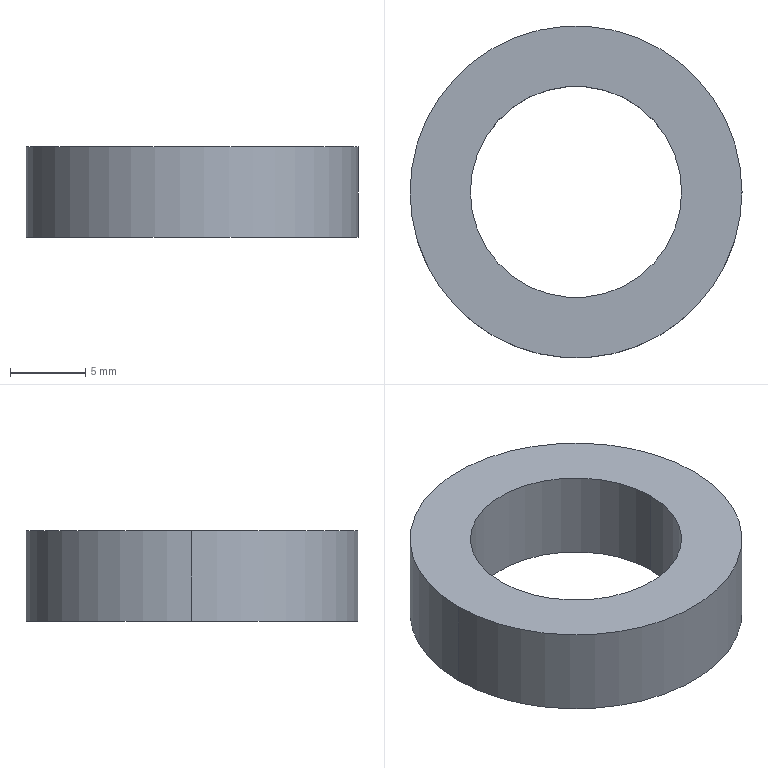Part | SolidWorks | features Revolution 1 | 1 solid | 6 faces | box 22 x 22 x 6 mm | volume 1357 mm3 | cylinder 4 | plane 2 | commonest cylinder face diameters 14 x2 22 x2
STEP:
#1=CARTESIAN_POINT('',(11.,0.,-6.));
#2=VERTEX_POINT('',#1);
#3=CARTESIAN_POINT('',(-11.,0.,-6.));
#4=VERTEX_POINT('',#3);
#5=CARTESIAN_POINT('',(0.,0.,-6.));
#6=DIRECTION('',(0.,0.,1.));
#7=DIRECTION('',(1.,0.,0.));
#8=AXIS2_PLACEMENT_3D('',#5,#6,#7);
#9=CIRCLE('',#8,11.);
#10=EDGE_CURVE('',#2,#4,#9,.T.);
#11=ORIENTED_EDGE('',*,*,#10,.T.);
#12=CARTESIAN_POINT('',(-11.,0.,0.));
#13=VERTEX_POINT('',#12);
#14=CARTESIAN_POINT('',(-11.,0.,4.548));
#15=DIRECTION('',(0.,0.,1.));
#16=VECTOR('',#15,1000.);
#17=LINE('',#14,#16);
#18=EDGE_CURVE('',#4,#13,#17,.T.);
#19=ORIENTED_EDGE('',*,*,#18,.T.);
#20=CARTESIAN_POINT('',(11.,0.,0.));
#21=VERTEX_POINT('',#20);
#22=CARTESIAN_POINT('',(0.,0.,0.));
#23=DIRECTION('',(0.,0.,1.));
#24=DIRECTION('',(1.,0.,0.));
#25=AXIS2_PLACEMENT_3D('',#22,#23,#24);
#26=CIRCLE('',#25,11.);
#27=EDGE_CURVE('',#21,#13,#26,.T.);
#28=ORIENTED_EDGE('',*,*,#27,.F.);
#29=CARTESIAN_POINT('',(11.,0.,4.548));
#30=DIRECTION('',(0.,0.,1.));
#31=VECTOR('',#30,1000.);
#32=LINE('',#29,#31);
#33=EDGE_CURVE('',#2,#21,#32,.T.);
#34=ORIENTED_EDGE('',*,*,#33,.F.);
#35=EDGE_LOOP('',(#11,#19,#28,#34));
#36=FACE_OUTER_BOUND('',#35,.T.);
#37=CARTESIAN_POINT('',(0.,0.,4.548));
#38=DIRECTION('',(0.,0.,1.));
#39=DIRECTION('',(1.,0.,0.));
#40=AXIS2_PLACEMENT_3D('',#37,#38,#39);
#41=CYLINDRICAL_SURFACE('',#40,11.);
#42=ADVANCED_FACE('',(#36),#41,.T.);
#43=CARTESIAN_POINT('',(-7.,0.,-6.));
#44=VERTEX_POINT('',#43);
#45=CARTESIAN_POINT('',(7.,0.,-6.));
#46=VERTEX_POINT('',#45);
#47=CARTESIAN_POINT('',(0.,0.,-6.));
#48=DIRECTION('',(0.,0.,1.));
#49=DIRECTION('',(1.,0.,0.));
#50=AXIS2_PLACEMENT_3D('',#47,#48,#49);
#51=CIRCLE('',#50,7.);
#52=EDGE_CURVE('',#44,#46,#51,.T.);
#53=ORIENTED_EDGE('',*,*,#52,.F.);
#54=CARTESIAN_POINT('',(-7.,0.,0.));
#55=VERTEX_POINT('',#54);
#56=CARTESIAN_POINT('',(-7.,0.,4.548));
#57=DIRECTION('',(0.,0.,1.));
#58=VECTOR('',#57,1000.);
#59=LINE('',#56,#58);
#60=EDGE_CURVE('',#44,#55,#59,.T.);
#61=ORIENTED_EDGE('',*,*,#60,.T.);
#62=CARTESIAN_POINT('',(7.,0.,0.));
#63=VERTEX_POINT('',#62);
#64=CARTESIAN_POINT('',(0.,0.,0.));
#65=DIRECTION('',(0.,0.,1.));
#66=DIRECTION('',(1.,0.,0.));
#67=AXIS2_PLACEMENT_3D('',#64,#65,#66);
#68=CIRCLE('',#67,7.);
#69=EDGE_CURVE('',#55,#63,#68,.T.);
#70=ORIENTED_EDGE('',*,*,#69,.T.);
#71=CARTESIAN_POINT('',(7.,0.,4.548));
#72=DIRECTION('',(0.,0.,1.));
#73=VECTOR('',#72,1000.);
#74=LINE('',#71,#73);
#75=EDGE_CURVE('',#46,#63,#74,.T.);
#76=ORIENTED_EDGE('',*,*,#75,.F.);
#77=EDGE_LOOP('',(#53,#61,#70,#76));
#78=FACE_OUTER_BOUND('',#77,.T.);
#79=CARTESIAN_POINT('',(0.,0.,4.548));
#80=DIRECTION('',(0.,0.,1.));
#81=DIRECTION('',(1.,0.,0.));
#82=AXIS2_PLACEMENT_3D('',#79,#80,#81);
#83=CYLINDRICAL_SURFACE('',#82,7.);
#84=ADVANCED_FACE('',(#78),#83,.F.);
#85=ORIENTED_EDGE('',*,*,#60,.F.);
#86=CARTESIAN_POINT('',(0.,0.,-6.));
#87=DIRECTION('',(0.,0.,1.));
#88=DIRECTION('',(1.,0.,0.));
#89=AXIS2_PLACEMENT_3D('',#86,#87,#88);
#90=CIRCLE('',#89,7.);
#91=EDGE_CURVE('',#46,#44,#90,.T.);
#92=ORIENTED_EDGE('',*,*,#91,.F.);
#93=ORIENTED_EDGE('',*,*,#75,.T.);
#94=CARTESIAN_POINT('',(0.,0.,0.));
#95=DIRECTION('',(0.,0.,1.));
#96=DIRECTION('',(1.,0.,0.));
#97=AXIS2_PLACEMENT_3D('',#94,#95,#96);
#98=CIRCLE('',#97,7.);
#99=EDGE_CURVE('',#63,#55,#98,.T.);
#100=ORIENTED_EDGE('',*,*,#99,.T.);
#101=EDGE_LOOP('',(#85,#92,#93,#100));
#102=FACE_OUTER_BOUND('',#101,.T.);
#103=CARTESIAN_POINT('',(0.,0.,4.548));
#104=DIRECTION('',(0.,0.,1.));
#105=DIRECTION('',(1.,0.,0.));
#106=AXIS2_PLACEMENT_3D('',#103,#104,#105);
#107=CYLINDRICAL_SURFACE('',#106,7.);
#108=ADVANCED_FACE('',(#102),#107,.F.);
#109=ORIENTED_EDGE('',*,*,#99,.F.);
#110=ORIENTED_EDGE('',*,*,#69,.F.);
#111=EDGE_LOOP('',(#109,#110));
#112=FACE_BOUND('',#111,.T.);
#113=ORIENTED_EDGE('',*,*,#27,.T.);
#114=CARTESIAN_POINT('',(0.,0.,0.));
#115=DIRECTION('',(0.,0.,1.));
#116=DIRECTION('',(1.,0.,0.));
#117=AXIS2_PLACEMENT_3D('',#114,#115,#116);
#118=CIRCLE('',#117,11.);
#119=EDGE_CURVE('',#13,#21,#118,.T.);
#120=ORIENTED_EDGE('',*,*,#119,.T.);
#121=EDGE_LOOP('',(#113,#120));
#122=FACE_OUTER_BOUND('',#121,.T.);
#123=CARTESIAN_POINT('',(0.,7.,0.));
#124=DIRECTION('',(0.,0.,-1.));
#125=DIRECTION('',(-1.,0.,0.));
#126=AXIS2_PLACEMENT_3D('',#123,#124,#125);
#127=PLANE('',#126);
#128=ADVANCED_FACE('',(#112,#122),#127,.F.);
#129=ORIENTED_EDGE('',*,*,#18,.F.);
#130=CARTESIAN_POINT('',(0.,0.,-6.));
#131=DIRECTION('',(0.,0.,1.));
#132=DIRECTION('',(1.,0.,0.));
#133=AXIS2_PLACEMENT_3D('',#130,#131,#132);
#134=CIRCLE('',#133,11.);
#135=EDGE_CURVE('',#4,#2,#134,.T.);
#136=ORIENTED_EDGE('',*,*,#135,.T.);
#137=ORIENTED_EDGE('',*,*,#33,.T.);
#138=ORIENTED_EDGE('',*,*,#119,.F.);
#139=EDGE_LOOP('',(#129,#136,#137,#138));
#140=FACE_OUTER_BOUND('',#139,.T.);
#141=CARTESIAN_POINT('',(0.,0.,4.548));
#142=DIRECTION('',(0.,0.,1.));
#143=DIRECTION('',(1.,0.,0.));
#144=AXIS2_PLACEMENT_3D('',#141,#142,#143);
#145=CYLINDRICAL_SURFACE('',#144,11.);
#146=ADVANCED_FACE('',(#140),#145,.T.);
#147=ORIENTED_EDGE('',*,*,#10,.F.);
#148=ORIENTED_EDGE('',*,*,#135,.F.);
#149=EDGE_LOOP('',(#147,#148));
#150=FACE_OUTER_BOUND('',#149,.T.);
#151=ORIENTED_EDGE('',*,*,#91,.T.);
#152=ORIENTED_EDGE('',*,*,#52,.T.);
#153=EDGE_LOOP('',(#151,#152));
#154=FACE_BOUND('',#153,.T.);
#155=CARTESIAN_POINT('',(0.,11.,-6.));
#156=DIRECTION('',(0.,0.,1.));
#157=DIRECTION('',(1.,0.,0.));
#158=AXIS2_PLACEMENT_3D('',#155,#156,#157);
#159=PLANE('',#158);
#160=ADVANCED_FACE('',(#150,#154),#159,.F.);
#161=CLOSED_SHELL('',(#42,#84,#108,#128,#146,#160));
#162=MANIFOLD_SOLID_BREP('',#161);
#163=CARTESIAN_POINT('',(0.,0.,0.));
#164=DIRECTION('',(0.,0.,1.));
#165=DIRECTION('',(1.,0.,0.));
#166=AXIS2_PLACEMENT_3D('',#163,#164,#165);
#167=(LENGTH_UNIT()NAMED_UNIT(*)SI_UNIT(.MILLI.,.METRE.));
#168=UNCERTAINTY_MEASURE_WITH_UNIT(LENGTH_MEASURE(0.00001),#167,'','');
#169=(NAMED_UNIT(*)PLANE_ANGLE_UNIT()SI_UNIT($,.RADIAN.));
#170=(NAMED_UNIT(*)SI_UNIT($,.STERADIAN.)SOLID_ANGLE_UNIT());
#171=(GEOMETRIC_REPRESENTATION_CONTEXT(3)GLOBAL_UNCERTAINTY_ASSIGNED_CONTEXT((#168))GLOBAL_UNIT_ASSIGNED_CONTEXT((#167,#169,#170))REPRESENTATION_CONTEXT('',''));
#172=ADVANCED_BREP_SHAPE_REPRESENTATION('',(#162,#166),#171);